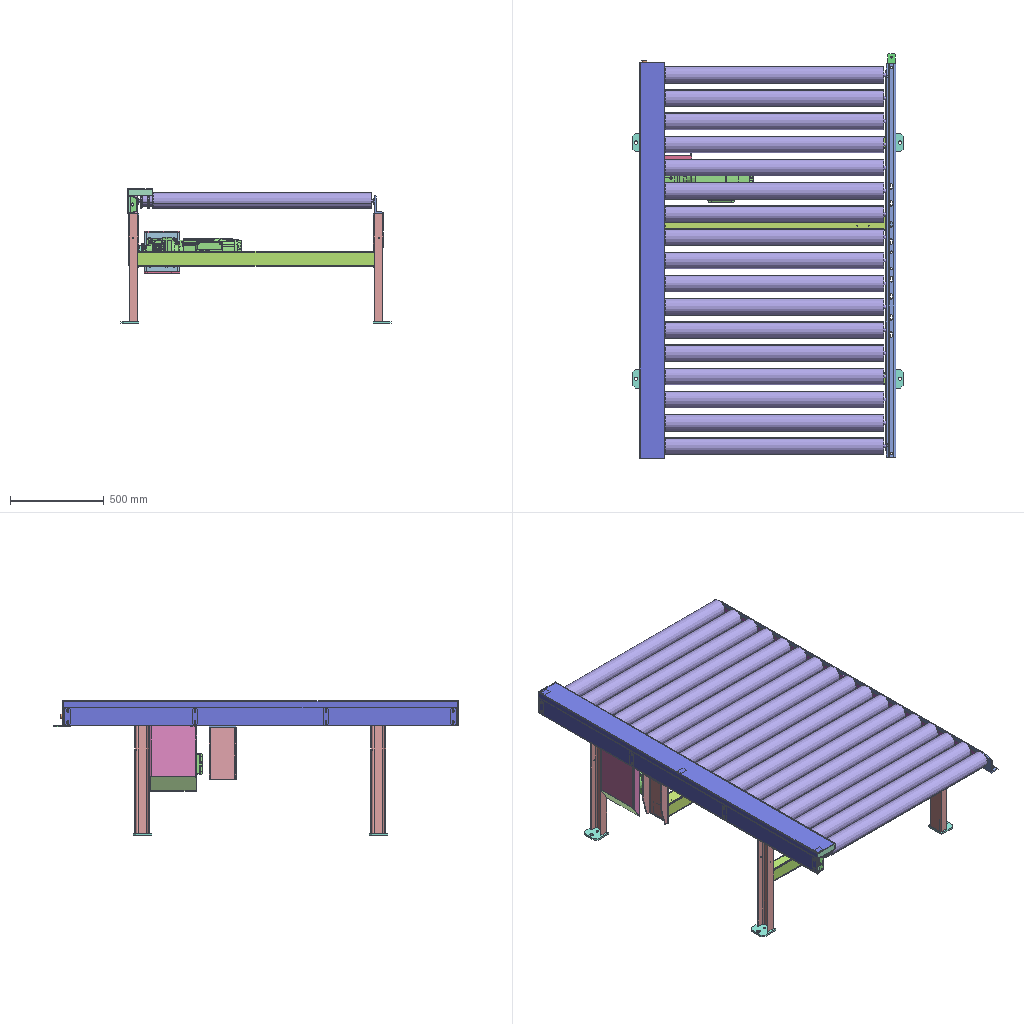Assembly | SolidWorks | 28 different items | 61 placed | box 1444 x 2158 x 720 mm
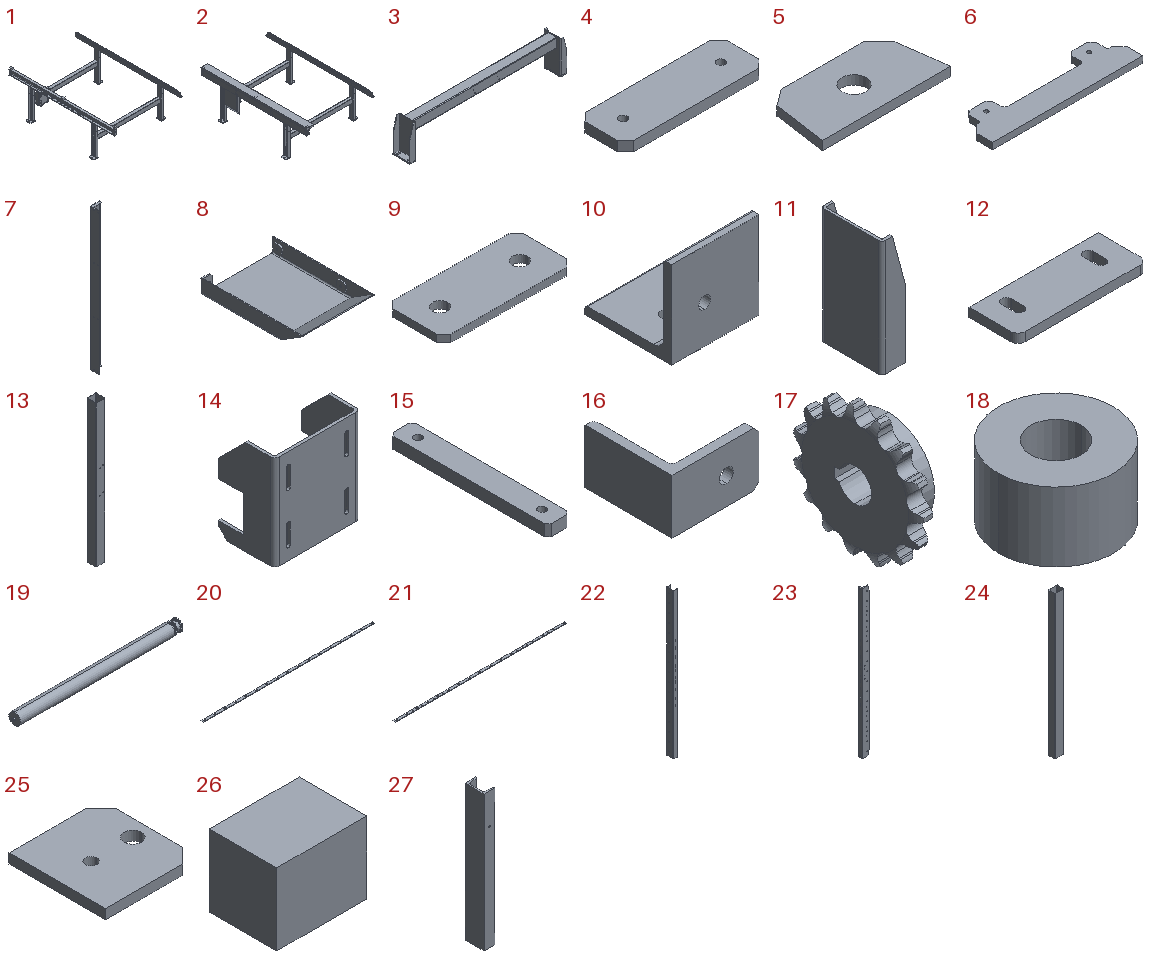Parts list (item | name | quantity | parent item | size | volume | features):
1 | (subassembly) | x1 | in 2 | 1444 x 2100 x 717 mm | 11597718 mm3 | features CompositeCurve 2
2 | (subassembly) | x1 | - | 1444 x 2158 x 720 mm | 13772315 mm3 | -
3 | (subassembly) | x1 | - | 1359 x 145 x 285 mm | 2027024 mm3 | -
4 | - | x4 | in 1 | 87 x 30 x 6 mm | 15124 mm3 | features Chamfer 1, Extrusion 1, ICE 1
5 | - | x2 | in 1 | 87 x 44 x 6 mm | 19570 mm3 | features Chamfer 1, Extrusion 1, ICE 1
6 | - | x2 | in 1 | 190 x 50 x 8 mm | 53772 mm3 | features Chamfer 1, Extrusion 1, Fillet 1, HoleWzd 1, ICE 1
7 | - | x1 | in 2 | 135 x 135 x 2110 mm | 1800450 mm3 | features FlatPattern 3, SMBaseFlange 3, SheetMetal 3, ICE 1
8 | - | x1 | in 2 | 250 x 350 x 50.917 mm | 357270 mm3 | features ICE 5, Chamfer 3, EdgeFlange 1, FlatPattern 1, HoleWzd 1, SMBaseFlange 1, SheetMetal 1
9 | - | x1 | in 2 | 90 x 40 x 5 mm | 16884 mm3 | features Extrusion 1
10 | - | x1 | - | 80 x 80 x 80 mm | 96906 mm3 | features ICE 2, WeldMemberFeat 1, WeldmentFeature 1
11 | - | x2 | in 3 | 55 x 145 x 275 mm | 373708 mm3 | features Extrusion 1, ICE 1
12 | - | x2 | in 3 | 145 x 55 x 10 mm | 74495 mm3 | features Extrusion 1, Fillet 1, ICE 1
13 | - | x1 | in 3 | 80 x 80 x 1249 mm | 1130618 mm3 | features HoleWzd 3, Extrusion 1, Fillet 1, Shell 1
14 | - | x1 | in 1 | 190 x 125 x 210 mm | 444526 mm3 | features Chamfer 2, ICE 2, Extrusion 1
15 | - | x2 | - | 20 x 140 x 10 mm | 27094 mm3 | features Chamfer 1, Extrusion 1, HoleWzd 1
16 | - | x1 | - | 80 x 80 x 50 mm | 59312 mm3 | features Fillet 3, Chamfer 1, Extrusion 1, ICE 1
17 | - | x1 | - | 25 x 98.203 x 98.722 mm | 107123 mm3 | features ICE 5, Chamfer 3, Cut 2, Revolution 2, CirPattern 1
18 | - | x1 | - | 25 x 25 x 15 mm | 5938 mm3 | features Extrusion 1
19 | - | x17 | - | 1264 x 89 x 89 mm | 7497180 mm3 | features ICE 6, MoveFace 6, HoleWzd 2, BaseBody 1, Chamfer 1
20 | - | x1 | in 1 | 2030 x 30 x 4 mm | 219056 mm3 | features Extrusion 1, Fillet 1, ICE 1
21 | - | x1 | in 1 | 2030 x 30 x 4 mm | 216015 mm3 | features ICE 2, Extrusion 1, Fillet 1
22 | - | x1 | in 1 | 50 x 100 x 2100 mm | 2750489 mm3 | features ICE 2, Extrusion 1
23 | - | x1 | in 1 | 100 x 50 x 2100 mm | 2805771 mm3 | features Fillet 2, ICE 2, Extrusion 1
24 | - | x2 | in 1 | 80 x 60 x 1264 mm | 993470 mm3 | features Extrusion 1, Fillet 1, Shell 1
25 | - | x4 | in 1 | 95 x 100 x 10 mm | 89074 mm3 | features Extrusion 1
26 | - | x3 | in 1 | 40 x 30 x 32 mm | 38400 mm3 | features Extrusion 1
27 | - | x4 | in 1 | 45 x 80 x 575 mm | 624060 mm3 | features Extrusion 1, HoleWzd 1
28 | R37DRN80M2BE1_20250626_055756_xB2AIP4sP02bcImaLGbvmg.stp | x1 | - | - | - | -
Mates (type | each side: item.copy, entity, surface, feature):
In the top assembly
Coincident | 19.1 face plane QCH21-D89-W1182-t3-d20 | 19.2 face plane QCH21-D89-W1182-t3-d20
Coincident | 19.3 face plane QCH21-D89-W1182-t3-d20 | 19.1 face plane QCH21-D89-W1182-t3-d20
Coincident | 19.4 face plane QCH21-D89-W1182-t3-d20 | 19.3 face plane QCH21-D89-W1182-t3-d20
Coincident | 19.4 face plane QCH21-D89-W1182-t3-d20 | 19.5 face plane QCH21-D89-W1182-t3-d20
Coincident | 19.5 face plane QCH21-D89-W1182-t3-d20 | 19.6 face plane QCH21-D89-W1182-t3-d20
Coincident | 19.7 face plane QCH21-D89-W1182-t3-d20 | 19.6 face plane QCH21-D89-W1182-t3-d20
Coincident | 19.8 face plane QCH21-D89-W1182-t3-d20 | 19.7 face plane QCH21-D89-W1182-t3-d20
Coincident | 19.9 face plane QCH21-D89-W1182-t3-d20 | 19.8 face plane QCH21-D89-W1182-t3-d20
Coincident | 19.9 face plane QCH21-D89-W1182-t3-d20 | 19.10 face plane QCH21-D89-W1182-t3-d20
Coincident | 19.11 face plane QCH21-D89-W1182-t3-d20 | 19.10 face plane QCH21-D89-W1182-t3-d20
Coincident | 19.12 face plane QCH21-D89-W1182-t3-d20 | 19.13 face plane QCH21-D89-W1182-t3-d20
Coincident | 19.14 face plane QCH21-D89-W1182-t3-d20 | 19.15 face plane QCH21-D89-W1182-t3-d20
Coincident | 19.16 face plane QCH21-D89-W1182-t3-d20 | 19.17 face plane QCH21-D89-W1182-t3-d20
Coincident | 19.14 face plane QCH21-D89-W1182-t3-d20 | 19.16 face plane QCH21-D89-W1182-t3-d20
Coincident | 19.12 face plane QCH21-D89-W1182-t3-d20 | 19.15 face plane QCH21-D89-W1182-t3-d20
Coincident | 19.11 face plane QCH21-D89-W1182-t3-d20 | 19.15 face plane QCH21-D89-W1182-t3-d20
Coincident | 23.1 face plane Boss-Extrude 1 | 19.17 face plane Boss-Extrude 2
Concentric | 23.1 face cylinder Cut-Extrude 1 | 19.17 face cylinder QCH21-D89-W1182-t3-d20
Concentric | 23.1 face cylinder Cut-Extrude 1 | 19.14 face cylinder QCH21-D89-W1182-t3-d20
Concentric | 23.1 face cylinder Cut-Extrude 1 | 19.16 face cylinder QCH21-D89-W1182-t3-d20
Concentric | 23.1 face cylinder Cut-Extrude 1 | 19.10 face cylinder QCH21-D89-W1182-t3-d20
Concentric | 23.1 face cylinder Cut-Extrude 1 | 19.9 face cylinder QCH21-D89-W1182-t3-d20
Concentric | 23.1 edge | 19.8 face cylinder QCH21-D89-W1182-t3-d20
Concentric | 23.1 face cylinder Cut-Extrude 1 | 19.15 face cylinder QCH21-D89-W1182-t3-d20
Concentric | 23.1 face cylinder Cut-Extrude 1 | 19.7 face cylinder QCH21-D89-W1182-t3-d20
Concentric | 23.1 face cylinder Cut-Extrude 1 | 19.6 face cylinder QCH21-D89-W1182-t3-d20
Concentric | 23.1 face cylinder Cut-Extrude 1 | 19.5 face cylinder QCH21-D89-W1182-t3-d20
Concentric | 23.1 face cylinder Cut-Extrude 1 | 19.4 face cylinder QCH21-D89-W1182-t3-d20
Concentric | 23.1 face cylinder Cut-Extrude 1 | 19.11 face cylinder QCH21-D89-W1182-t3-d20
Concentric | 23.1 face cylinder Cut-Extrude 1 | 19.12 face cylinder QCH21-D89-W1182-t3-d20
Concentric | 23.1 face cylinder Cut-Extrude 1 | 19.13 face cylinder QCH21-D89-W1182-t3-d20
Concentric | 23.1 face cylinder Cut-Extrude 1 | 19.3 face cylinder QCH21-D89-W1182-t3-d20
Concentric | 23.1 face cylinder Cut-Extrude 1 | 19.1 face cylinder QCH21-D89-W1182-t3-d20
Concentric | 23.1 face cylinder Cut-Extrude 1 | 19.2 face cylinder QCH21-D89-W1182-t3-d20
Coincident | 14.1 face plane Boss-Extrude 1 | 15.1 face plane Boss-Extrude 1
Slot | 15.1 face cylinder M8 Tapped Hole 1 | 14.1 face cylinder Cut-Extrude 1
Parallel | 14.1 face plane Boss-Extrude 1 | 15.1 face plane Boss-Extrude 1
Coincident | 15.1 face plane Boss-Extrude 1 | 15.2 face plane Boss-Extrude 1 | 2 times
Slot | 15.2 face cylinder M8 Tapped Hole 1 | 14.1 face plane Cut-Extrude 1
Concentric | 5.1 face cylinder Cut-Extrude 1 | 18.1 face cylinder Boss-Extrude 1
Coincident | 5.1 face plane Boss-Extrude 1 | 18.1 face plane Boss-Extrude 1
Coincident | 23.1 face plane Boss-Extrude 1 | 12.1 face plane Boss-Extrude 1
Width | 12.2 face plane Boss-Extrude 1 | 12.1 face plane Boss-Extrude 1 | 22.1 face plane Boss-Extrude 1 | 23.1 face plane Boss-Extrude 1
In subassembly 3
Coincident | 11.1 face plane Boss-Extrude 1 | 13.1 face plane Boss-Extrude 1
Coincident | 13.1 face plane Boss-Extrude 1 | 11.2 face plane Boss-Extrude 1
Coincident | 11.1 face plane Boss-Extrude 1 | 11.2 face plane Boss-Extrude 1 | 2 times
DistanceDim | 13.1 face plane Boss-Extrude 1 | 11.1 face plane Boss-Extrude 1
DistanceDim | 11.1 face plane Boss-Extrude 1 | 13.1 face plane Boss-Extrude 1
Coincident | 11.1 face plane Boss-Extrude 1 | 12.3 face plane Boss-Extrude 1 | 2 times
Concentric | 11.1 face cylinder Boss-Extrude 1 | 12.3 face cylinder Fillet 1
Coincident | 11.2 face plane Boss-Extrude 1 | 12.4 face plane Boss-Extrude 1 | 2 times
Concentric | 11.2 face cylinder Boss-Extrude 1 | 12.4 face cylinder Fillet 1
In subassembly 2
Coincident | 22.2 face plane Boss-Extrude 1 | 7.1 face plane Base-Flange 2
Coincident | 22.2 face plane Boss-Extrude 1 | 7.1 face plane Base-Flange 1
Width | 7.1 face plane Base-Flange 2 | 7.1 face plane Base-Flange 3 | 22.2 face plane Boss-Extrude 1 | 22.2 face plane Boss-Extrude 1
Coincident | 27.1 face plane Boss-Extrude 1 | 8.1 face plane Edge-Flange 1
Coincident | 22.2 face plane Boss-Extrude 1 | 8.1 face plane Boss-Extrude 7 | 2 times
Coincident | 23.2 face plane Boss-Extrude 1 | 9.1 face plane Boss-Extrude 1
Parallel | 23.2 face plane Boss-Extrude 1 | 9.1 face plane Boss-Extrude 1
Concentric | 23.2 face cylinder Cut-Extrude 2 | 9.1 face cylinder Boss-Extrude 1
In subassembly 1
Coincident | 27.2 face plane Boss-Extrude 1 | 27.3 face plane Boss-Extrude 1 | 2 times
Coincident | 27.3 face plane Boss-Extrude 1 | 27.4 face plane Boss-Extrude 1 | 2 times
Parallel | 27.2 face plane Boss-Extrude 1 | 27.5 face plane Boss-Extrude 1
Coincident | 27.2 face plane Boss-Extrude 1 | 27.5 face plane Boss-Extrude 1 | 2 times
Coincident | 27.5 face plane Boss-Extrude 1 | 27.4 face plane Boss-Extrude 1
Coincident | 27.2 face plane Boss-Extrude 1 | 24.1 face plane Boss-Extrude 1
Coincident | 27.3 face plane Boss-Extrude 1 | 24.1 edge
Width | 24.1 face plane Boss-Extrude 1 | 24.1 face plane Boss-Extrude 1 | 27.3 face plane Boss-Extrude 1 | 27.3 face plane Boss-Extrude 1
Coincident | 27.4 face plane Boss-Extrude 1 | 24.2 face plane Boss-Extrude 1
Coincident | 24.1 face plane Boss-Extrude 1 | 24.2 face plane Boss-Extrude 1
Width | 24.2 face plane Boss-Extrude 1 | 24.2 face plane Boss-Extrude 1 | 27.5 face plane Boss-Extrude 1 | 27.5 face plane Boss-Extrude 1
DistanceDim | 27.4 face plane Boss-Extrude 1 | 27.3 face plane Boss-Extrude 1
Coincident | 27.5 face plane Boss-Extrude 1 | 23.3 face plane Boss-Extrude 1
Width | 23.3 face plane Boss-Extrude 1 | 23.3 face plane Boss-Extrude 1 | 27.2 face plane Boss-Extrude 1 | 27.5 face plane Boss-Extrude 1
Coincident | 27.2 face plane Boss-Extrude 1 | 23.3 face plane Boss-Extrude 1
Coincident | 27.3 face plane Boss-Extrude 1 | 22.3 face plane Boss-Extrude 1
Coincident | 27.4 face plane Boss-Extrude 1 | 22.3 face plane Boss-Extrude 1
Width | 22.3 face plane Boss-Extrude 1 | 22.3 face plane Boss-Extrude 1 | 27.3 face plane Boss-Extrude 1 | 27.4 face plane Boss-Extrude 1
DistanceDim | 24.2 face plane Boss-Extrude 1 | 23.3 face plane Boss-Extrude 1
DistanceDim | 25.1 face plane Boss-Extrude 1 | 27.5 face plane Boss-Extrude 1
Coincident | 27.5 face plane Boss-Extrude 1 | 25.1 face plane Boss-Extrude 1
Width | 25.1 face plane Boss-Extrude 1 | 25.1 face plane Boss-Extrude 1 | 27.5 face plane Boss-Extrude 1 | 27.5 face plane Boss-Extrude 1
Coincident | 25.2 face plane Boss-Extrude 1 | 25.3 face plane Boss-Extrude 1 | 2 times
Coincident | 25.4 face plane Boss-Extrude 1 | 25.3 face plane Boss-Extrude 1
Coincident | 25.1 face plane Boss-Extrude 1 | 25.4 face plane Boss-Extrude 1 | 2 times
Coincident | 25.4 face plane Boss-Extrude 1 | 25.2 face plane Boss-Extrude 1
DistanceDim | 27.4 face plane Boss-Extrude 1 | 25.4 face plane Boss-Extrude 1
Coincident | 25.1 face plane Boss-Extrude 1 | 25.3 face plane Boss-Extrude 1
Width | 25.2 face plane Boss-Extrude 1 | 25.2 face plane Boss-Extrude 1 | 27.3 face plane Boss-Extrude 1 | 27.3 face plane Boss-Extrude 1
Coincident | 26.1 face plane Boss-Extrude 1 | 26.2 face plane Boss-Extrude 1
Coincident | 26.2 face plane Boss-Extrude 1 | 26.3 face plane Boss-Extrude 1 | 2 times
Coincident | 26.1 face plane Boss-Extrude 1 | 26.3 face plane Boss-Extrude 1
Coincident | 22.3 face plane Boss-Extrude 1 | 26.2 face plane Boss-Extrude 1
DistanceDim | 26.3 face plane Boss-Extrude 1 | 26.2 face plane Boss-Extrude 1
Width | 26.2 face plane Boss-Extrude 1 | 26.3 face plane Boss-Extrude 1 | 22.3 face plane Boss-Extrude 1 | 22.3 face plane Boss-Extrude 1
DistanceDim | 26.2 face plane Boss-Extrude 1 | 26.1 face plane Boss-Extrude 1
Coincident | 4.1 face plane Boss-Extrude 1 | 4.2 face plane Boss-Extrude 1 | 2 times
Coincident | 4.1 face plane Boss-Extrude 1 | 4.3 face plane Boss-Extrude 1 | 2 times
Coincident | 4.4 face plane Boss-Extrude 1 | 4.1 face plane Boss-Extrude 1
Coincident | 4.4 face plane Boss-Extrude 1 | 4.3 face plane Boss-Extrude 1
Width | 22.3 face plane Boss-Extrude 1 | 22.3 face plane Boss-Extrude 1 | 4.1 face plane Boss-Extrude 1 | 4.1 face plane Boss-Extrude 1
Parallel | 22.3 face plane Boss-Extrude 1 | 4.1 face plane Boss-Extrude 1
Coincident | 22.3 face plane Boss-Extrude 1 | 5.2 face plane Boss-Extrude 1 | 2 times
Width | 5.2 face plane Cut-Extrude 1 | 5.2 face plane Cut-Extrude 1 | 22.3 face plane Boss-Extrude 1 | 22.3 face plane Boss-Extrude 1
Coincident | 4.2 face plane Boss-Extrude 1 | 5.2 face plane Boss-Extrude 1 | 2 times
Coincident | 5.2 face plane Boss-Extrude 1 | 5.3 face plane Boss-Extrude 1
Coincident | 5.2 face plane Cut-Extrude 1 | 5.3 face plane Cut-Extrude 1
Coincident | 22.3 face plane Boss-Extrude 1 | 5.3 face plane Boss-Extrude 1
Coincident | 22.3 face plane Boss-Extrude 1 | 26.3 face plane Boss-Extrude 1
Coincident | 4.1 face plane Boss-Extrude 1 | 5.3 face plane Boss-Extrude 1
Coincident | 24.1 face plane Boss-Extrude 1 | 14.2 face plane Cut-Extrude 2 | 2 times
Coincident | 6.1 face plane Boss-Extrude 1 | 14.2 face plane Boss-Extrude 1 | 2 times
Coincident | 6.1 face plane Cut-Extrude 1 | 14.2 face plane Boss-Extrude 1
DistanceDim | 27.3 face plane Boss-Extrude 1 | 14.2 face plane Boss-Extrude 1
DistanceDim | 4.2 face plane Boss-Extrude 1 | 4.3 face plane Boss-Extrude 1
DistanceDim | 4.4 face plane Boss-Extrude 1 | 4.3 face plane Boss-Extrude 1
Coincident | 22.3 face plane Boss-Extrude 1 | 20.1 face plane Boss-Extrude 1
Concentric | 22.3 face cylinder Cut-Extrude 1 | 20.1 face cylinder Cut-Extrude 1 | 2 times
Coincident | 23.3 face plane Boss-Extrude 1 | 21.1 face plane Boss-Extrude 1
Concentric | 23.3 edge | 21.1 face cylinder Cut-Extrude 1
Concentric | 23.3 face cylinder Cut-Extrude 1 | 21.1 face cylinder Cut-Extrude 1
Coincident | 6.1 face plane Boss-Extrude 1 | 6.2 face plane Boss-Extrude 1 | 2 times
Coincident | 14.2 face plane Boss-Extrude 1 | 6.2 face plane Boss-Extrude 1